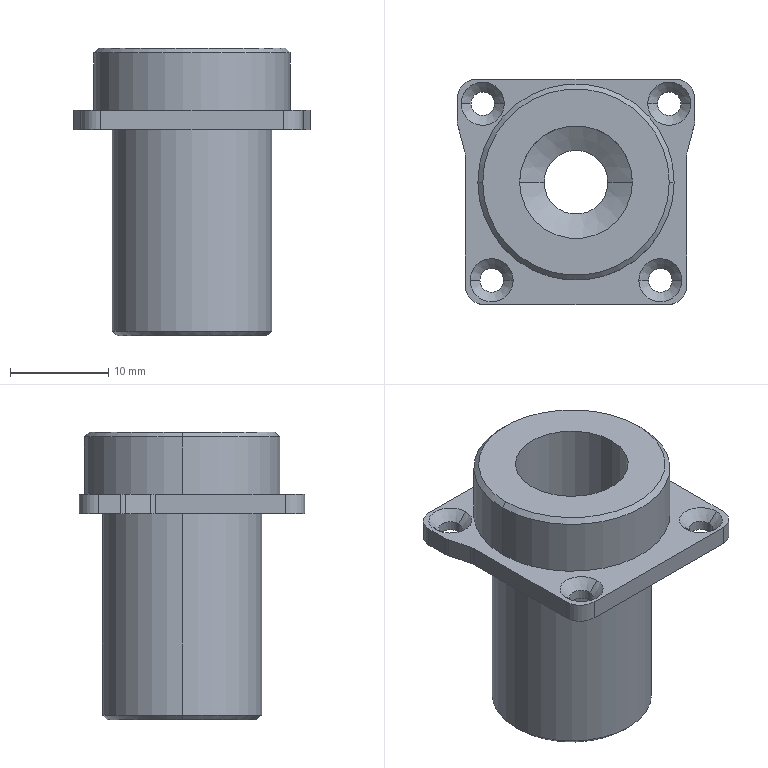Part | 1 solid | 70 faces | box 24.2 x 23 x 29.342 mm | volume 4442 mm3 | cylinder 30 | cone 20 | plane 14 | torus 6 | commonest cylinder face diameters 2.4 x8 4 x8 6.5 x2 8.17 x2 11.15 x2 11.5 x2